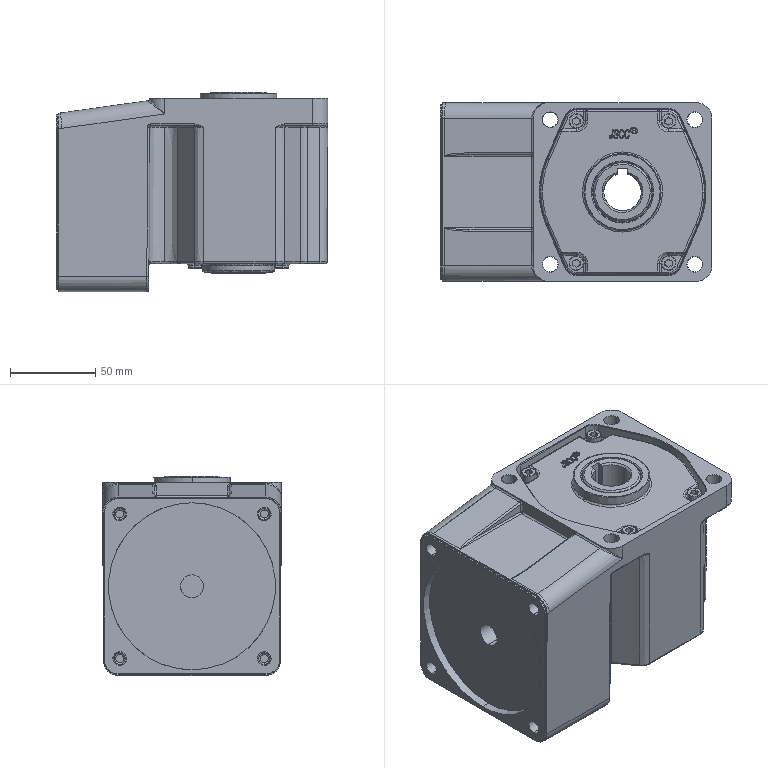Part | STEP file | 11-100GF-RC11 | 1 solid | 897 faces | box 159.399 x 104.797 x 116.9 mm | volume 1389549 mm3 | cylinder 302 | plane 211 | spline 153 | torus 133 | cone 75 | sphere 23 | commonest cylinder face diameters 2 x87 0.5 x28 1 x26 5 x16 18 x12 8 x11